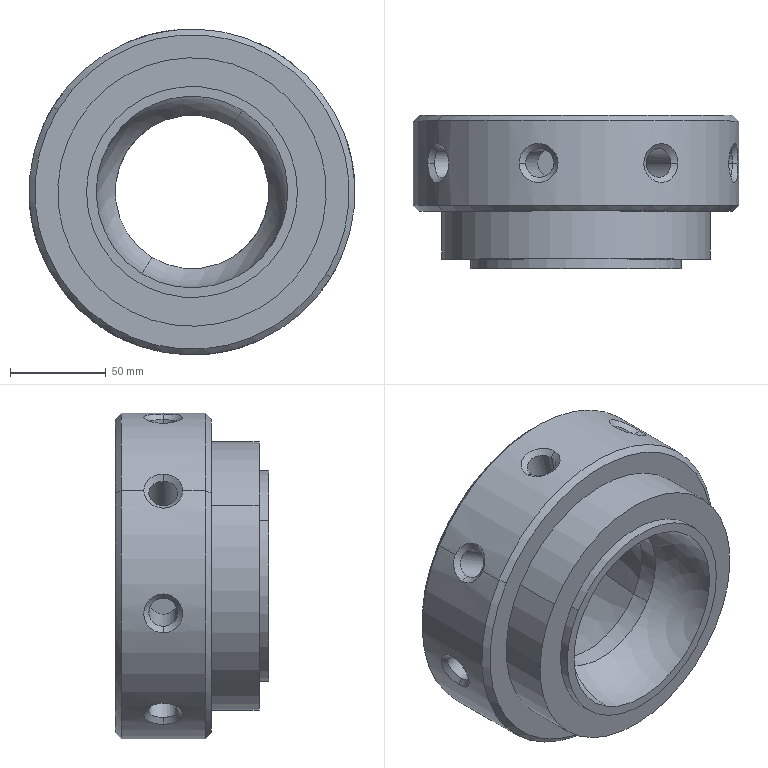Part | SolidWorks | features BaseBody 1 | 1 solid | 68 faces | box 170 x 80 x 170 mm | volume 1005537 mm3 | cylinder 24 | spline 24 | plane 12 | cone 6 | sphere 2 | commonest cylinder face diameters 15 x16 80 x2 110 x2 140 x2 170 x2